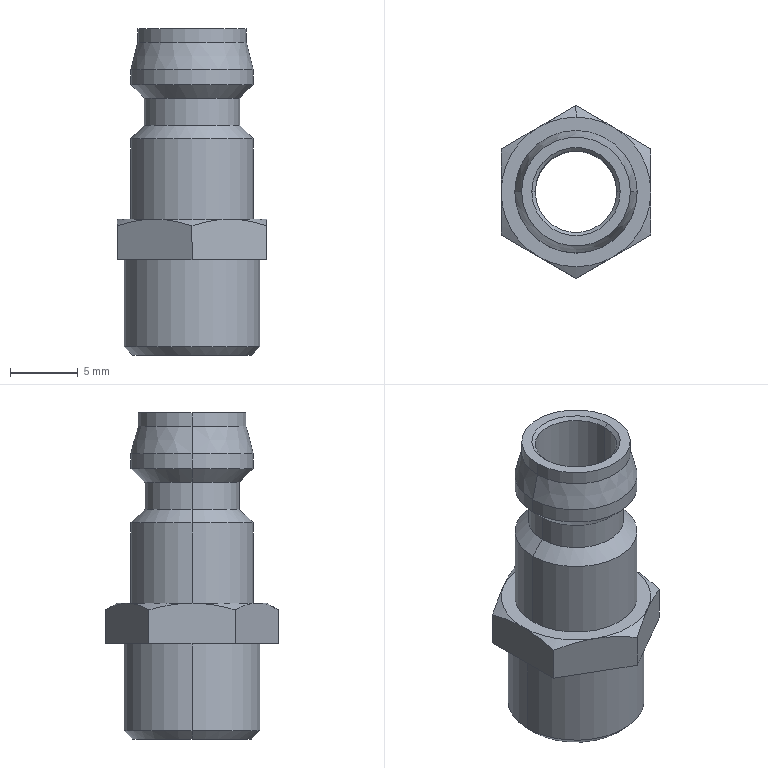Part | STEP file | KH-060 ENM 10 | 1 solid | 41 faces | box 11 x 12.702 x 24 mm | volume 962.573 mm3 | cone 19 | cylinder 12 | plane 10 | commonest cylinder face diameters 9 x4 6 x2 7 x2 8 x2 10 x2